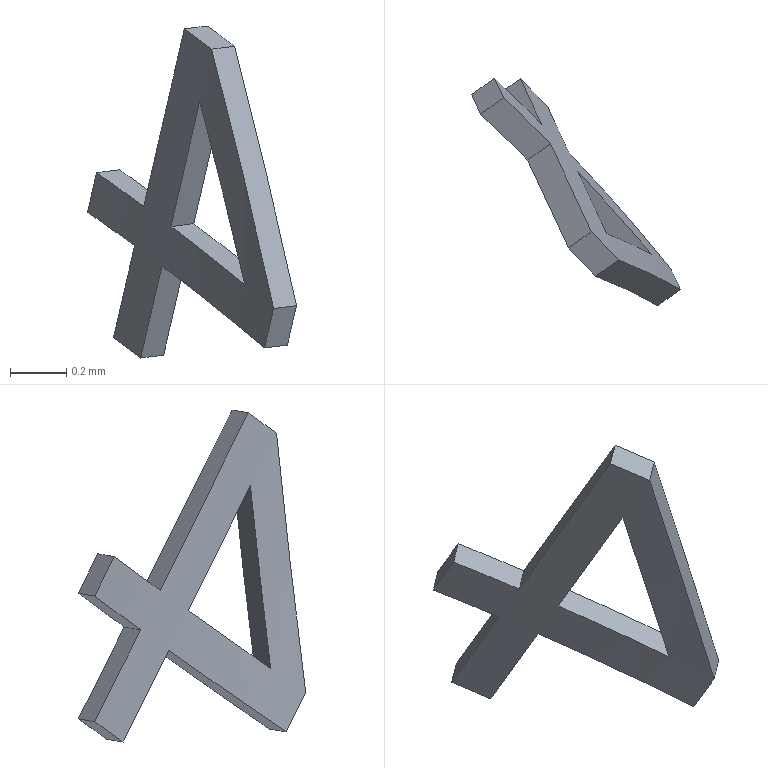Part | SolidWorks | features BaseBody 1 | 1 solid | 16 faces | box 0.7417 x 0.8074 x 1.179 mm | volume 0.04503 mm3 | plane 14 | cylinder 2 | commonest cylinder face diameters 16.8 x1 17 x1
STEP:
#1=CARTESIAN_POINT('',(1972.672,-237.776,993.123));
#2=VERTEX_POINT('',#1);
#3=CARTESIAN_POINT('',(1972.747,-237.939,993.449));
#4=VERTEX_POINT('',#3);
#5=CARTESIAN_POINT('',(1973.875,-240.379,998.359));
#6=DIRECTION('',(0.2015,-0.436,0.8771));
#7=VECTOR('',#6,1000.);
#8=LINE('',#5,#7);
#9=EDGE_CURVE('',#2,#4,#8,.T.);
#10=ORIENTED_EDGE('',*,*,#9,.T.);
#11=CARTESIAN_POINT('',(1973.112,-238.355,993.158));
#12=VERTEX_POINT('',#11);
#13=CARTESIAN_POINT('',(1966.322,-243.225,992.297));
#14=DIRECTION('',(-0.2015,0.436,-0.8771));
#15=DIRECTION('',(-0.7309,-0.6631,-0.1618));
#16=AXIS2_PLACEMENT_3D('',#13,#14,#15);
#17=CIRCLE('',#16,8.4);
#18=EDGE_CURVE('',#4,#12,#17,.T.);
#19=ORIENTED_EDGE('',*,*,#18,.T.);
#20=CARTESIAN_POINT('',(1973.144,-238.425,993.298));
#21=VERTEX_POINT('',#20);
#22=CARTESIAN_POINT('',(1974.24,-240.796,998.068));
#23=DIRECTION('',(0.2015,-0.436,0.8771));
#24=VECTOR('',#23,1000.);
#25=LINE('',#22,#24);
#26=EDGE_CURVE('',#12,#21,#25,.T.);
#27=ORIENTED_EDGE('',*,*,#26,.T.);
#28=CARTESIAN_POINT('',(1972.924,-238.321,994.219));
#29=VERTEX_POINT('',#28);
#30=CARTESIAN_POINT('',(1972.924,-238.321,994.219));
#31=CARTESIAN_POINT('',(1973.004,-238.351,993.913));
#32=CARTESIAN_POINT('',(1973.077,-238.386,993.606));
#33=CARTESIAN_POINT('',(1973.144,-238.425,993.298));
#34=B_SPLINE_CURVE_WITH_KNOTS('',3,(#30,#31,#32,#33),.UNSPECIFIED.,.F.,.F.,(4,4),(0.,1.),.UNSPECIFIED.);
#35=EDGE_CURVE('',#29,#21,#34,.T.);
#36=ORIENTED_EDGE('',*,*,#35,.F.);
#37=CARTESIAN_POINT('',(1972.827,-238.221,994.291));
#38=VERTEX_POINT('',#37);
#39=CARTESIAN_POINT('',(1966.499,-243.608,993.067));
#40=DIRECTION('',(0.2015,-0.436,0.8771));
#41=DIRECTION('',(-0.7309,-0.6631,-0.1618));
#42=AXIS2_PLACEMENT_3D('',#39,#40,#41);
#43=CIRCLE('',#42,8.4);
#44=EDGE_CURVE('',#29,#38,#43,.T.);
#45=ORIENTED_EDGE('',*,*,#44,.T.);
#46=CARTESIAN_POINT('',(1972.683,-237.908,993.661));
#47=VERTEX_POINT('',#46);
#48=CARTESIAN_POINT('',(1973.778,-240.28,998.431));
#49=DIRECTION('',(-0.2015,0.436,-0.8771));
#50=VECTOR('',#49,1000.);
#51=LINE('',#48,#50);
#52=EDGE_CURVE('',#38,#47,#51,.T.);
#53=ORIENTED_EDGE('',*,*,#52,.T.);
#54=CARTESIAN_POINT('',(1972.515,-237.746,993.781));
#55=VERTEX_POINT('',#54);
#56=CARTESIAN_POINT('',(1966.354,-243.295,992.437));
#57=DIRECTION('',(0.2015,-0.436,0.8771));
#58=DIRECTION('',(-0.7309,-0.6631,-0.1618));
#59=AXIS2_PLACEMENT_3D('',#56,#57,#58);
#60=CIRCLE('',#59,8.4);
#61=EDGE_CURVE('',#47,#55,#60,.T.);
#62=ORIENTED_EDGE('',*,*,#61,.T.);
#63=CARTESIAN_POINT('',(1972.483,-237.676,993.641));
#64=VERTEX_POINT('',#63);
#65=CARTESIAN_POINT('',(1973.611,-240.117,998.55));
#66=DIRECTION('',(-0.2015,0.436,-0.8771));
#67=VECTOR('',#66,1000.);
#68=LINE('',#65,#67);
#69=EDGE_CURVE('',#55,#64,#68,.T.);
#70=ORIENTED_EDGE('',*,*,#69,.T.);
#71=CARTESIAN_POINT('',(1972.65,-237.839,993.521));
#72=VERTEX_POINT('',#71);
#73=CARTESIAN_POINT('',(1966.322,-243.225,992.297));
#74=DIRECTION('',(-0.2015,0.436,-0.8771));
#75=DIRECTION('',(-0.7309,-0.6631,-0.1618));
#76=AXIS2_PLACEMENT_3D('',#73,#74,#75);
#77=CIRCLE('',#76,8.4);
#78=EDGE_CURVE('',#64,#72,#77,.T.);
#79=ORIENTED_EDGE('',*,*,#78,.T.);
#80=CARTESIAN_POINT('',(1972.575,-237.676,993.195));
#81=VERTEX_POINT('',#80);
#82=CARTESIAN_POINT('',(1973.778,-240.28,998.431));
#83=DIRECTION('',(-0.2015,0.436,-0.8771));
#84=VECTOR('',#83,1000.);
#85=LINE('',#82,#84);
#86=EDGE_CURVE('',#72,#81,#85,.T.);
#87=ORIENTED_EDGE('',*,*,#86,.T.);
#88=CARTESIAN_POINT('',(1966.247,-243.063,991.97));
#89=DIRECTION('',(-0.2015,0.436,-0.8771));
#90=DIRECTION('',(-0.7309,-0.6631,-0.1618));
#91=AXIS2_PLACEMENT_3D('',#88,#89,#90);
#92=CIRCLE('',#91,8.4);
#93=EDGE_CURVE('',#81,#2,#92,.T.);
#94=ORIENTED_EDGE('',*,*,#93,.T.);
#95=EDGE_LOOP('',(#10,#19,#27,#36,#45,#53,#62,#70,#79,#87,#94));
#96=FACE_OUTER_BOUND('',#95,.T.);
#97=CARTESIAN_POINT('',(1972.881,-238.229,994.032));
#98=VERTEX_POINT('',#97);
#99=CARTESIAN_POINT('',(1973.042,-238.301,993.384));
#100=VERTEX_POINT('',#99);
#101=CARTESIAN_POINT('',(1972.881,-238.229,994.032));
#102=CARTESIAN_POINT('',(1972.938,-238.25,993.817));
#103=CARTESIAN_POINT('',(1972.991,-238.274,993.6));
#104=CARTESIAN_POINT('',(1973.042,-238.301,993.384));
#105=B_SPLINE_CURVE_WITH_KNOTS('',3,(#101,#102,#103,#104),.UNSPECIFIED.,.F.,.F.,(4,4),(0.,1.),.UNSPECIFIED.);
#106=EDGE_CURVE('',#98,#100,#105,.T.);
#107=ORIENTED_EDGE('',*,*,#106,.T.);
#108=CARTESIAN_POINT('',(1972.78,-238.008,993.589));
#109=VERTEX_POINT('',#108);
#110=CARTESIAN_POINT('',(1966.354,-243.295,992.437));
#111=DIRECTION('',(0.2015,-0.436,0.8771));
#112=DIRECTION('',(-0.7309,-0.6631,-0.1618));
#113=AXIS2_PLACEMENT_3D('',#110,#111,#112);
#114=CIRCLE('',#113,8.4);
#115=EDGE_CURVE('',#100,#109,#114,.T.);
#116=ORIENTED_EDGE('',*,*,#115,.T.);
#117=CARTESIAN_POINT('',(1973.875,-240.379,998.359));
#118=DIRECTION('',(0.2015,-0.436,0.8771));
#119=VECTOR('',#118,1000.);
#120=LINE('',#117,#119);
#121=EDGE_CURVE('',#109,#98,#120,.T.);
#122=ORIENTED_EDGE('',*,*,#121,.T.);
#123=EDGE_LOOP('',(#107,#116,#122));
#124=FACE_BOUND('',#123,.T.);
#125=CARTESIAN_POINT('',(1967.45,-245.666,997.207));
#126=DIRECTION('',(0.2015,-0.436,0.8771));
#127=DIRECTION('',(-0.7309,-0.6631,-0.1618));
#128=AXIS2_PLACEMENT_3D('',#125,#126,#127);
#129=CYLINDRICAL_SURFACE('',#128,8.4);
#130=ADVANCED_FACE('',(#96,#124),#129,.F.);
#131=CARTESIAN_POINT('',(1972.754,-237.718,993.133));
#132=VERTEX_POINT('',#131);
#133=CARTESIAN_POINT('',(1972.713,-237.747,993.128));
#134=DIRECTION('',(-0.8088,-0.5792,-0.1022));
#135=VECTOR('',#134,1000.);
#136=LINE('',#133,#135);
#137=EDGE_CURVE('',#132,#2,#136,.T.);
#138=ORIENTED_EDGE('',*,*,#137,.T.);
#139=ORIENTED_EDGE('',*,*,#93,.F.);
#140=CARTESIAN_POINT('',(1972.657,-237.618,993.205));
#141=VERTEX_POINT('',#140);
#142=CARTESIAN_POINT('',(1972.616,-237.647,993.2));
#143=DIRECTION('',(-0.8088,-0.5792,-0.1022));
#144=VECTOR('',#143,1000.);
#145=LINE('',#142,#144);
#146=EDGE_CURVE('',#141,#81,#145,.T.);
#147=ORIENTED_EDGE('',*,*,#146,.F.);
#148=CARTESIAN_POINT('',(1966.247,-243.063,991.97));
#149=DIRECTION('',(-0.2015,0.436,-0.8771));
#150=DIRECTION('',(-0.7309,-0.6631,-0.1618));
#151=AXIS2_PLACEMENT_3D('',#148,#149,#150);
#152=CIRCLE('',#151,8.5);
#153=EDGE_CURVE('',#141,#132,#152,.T.);
#154=ORIENTED_EDGE('',*,*,#153,.T.);
#155=EDGE_LOOP('',(#138,#139,#147,#154));
#156=FACE_OUTER_BOUND('',#155,.T.);
#157=CARTESIAN_POINT('',(1981.656,-238.46,990.719));
#158=DIRECTION('',(-0.2015,0.436,-0.8771));
#159=DIRECTION('',(-0.5526,0.6888,0.4693));
#160=AXIS2_PLACEMENT_3D('',#157,#158,#159);
#161=PLANE('',#160);
#162=ADVANCED_FACE('',(#156),#161,.T.);
#163=ORIENTED_EDGE('',*,*,#146,.T.);
#164=ORIENTED_EDGE('',*,*,#86,.F.);
#165=CARTESIAN_POINT('',(1972.732,-237.781,993.532));
#166=VERTEX_POINT('',#165);
#167=CARTESIAN_POINT('',(1972.691,-237.81,993.526));
#168=DIRECTION('',(-0.8088,-0.5792,-0.1022));
#169=VECTOR('',#168,1000.);
#170=LINE('',#167,#169);
#171=EDGE_CURVE('',#166,#72,#170,.T.);
#172=ORIENTED_EDGE('',*,*,#171,.F.);
#173=CARTESIAN_POINT('',(1972.694,-237.699,993.368));
#174=DIRECTION('',(-0.2015,0.436,-0.8771));
#175=VECTOR('',#174,1000.);
#176=LINE('',#173,#175);
#177=EDGE_CURVE('',#166,#141,#176,.T.);
#178=ORIENTED_EDGE('',*,*,#177,.T.);
#179=EDGE_LOOP('',(#163,#164,#172,#178));
#180=FACE_OUTER_BOUND('',#179,.T.);
#181=CARTESIAN_POINT('',(1978.018,-233.995,994.199));
#182=DIRECTION('',(-0.5526,0.6888,0.4693));
#183=DIRECTION('',(0.2015,-0.436,0.8771));
#184=AXIS2_PLACEMENT_3D('',#181,#182,#183);
#185=PLANE('',#184);
#186=ADVANCED_FACE('',(#180),#185,.T.);
#187=ORIENTED_EDGE('',*,*,#171,.T.);
#188=ORIENTED_EDGE('',*,*,#78,.F.);
#189=CARTESIAN_POINT('',(1972.565,-237.618,993.651));
#190=VERTEX_POINT('',#189);
#191=CARTESIAN_POINT('',(1972.524,-237.647,993.646));
#192=DIRECTION('',(-0.8088,-0.5792,-0.1022));
#193=VECTOR('',#192,1000.);
#194=LINE('',#191,#193);
#195=EDGE_CURVE('',#190,#64,#194,.T.);
#196=ORIENTED_EDGE('',*,*,#195,.F.);
#197=CARTESIAN_POINT('',(1966.322,-243.225,992.297));
#198=DIRECTION('',(-0.2015,0.436,-0.8771));
#199=DIRECTION('',(-0.7309,-0.6631,-0.1618));
#200=AXIS2_PLACEMENT_3D('',#197,#198,#199);
#201=CIRCLE('',#200,8.5);
#202=EDGE_CURVE('',#190,#166,#201,.T.);
#203=ORIENTED_EDGE('',*,*,#202,.T.);
#204=EDGE_LOOP('',(#187,#188,#196,#203));
#205=FACE_OUTER_BOUND('',#204,.T.);
#206=CARTESIAN_POINT('',(1977.874,-233.815,994.322));
#207=DIRECTION('',(-0.2015,0.436,-0.8771));
#208=DIRECTION('',(-0.5526,0.6888,0.4693));
#209=AXIS2_PLACEMENT_3D('',#206,#207,#208);
#210=PLANE('',#209);
#211=ADVANCED_FACE('',(#205),#210,.T.);
#212=ORIENTED_EDGE('',*,*,#195,.T.);
#213=ORIENTED_EDGE('',*,*,#69,.F.);
#214=CARTESIAN_POINT('',(1972.597,-237.687,993.791));
#215=VERTEX_POINT('',#214);
#216=CARTESIAN_POINT('',(1972.556,-237.716,993.786));
#217=DIRECTION('',(-0.8088,-0.5792,-0.1022));
#218=VECTOR('',#217,1000.);
#219=LINE('',#216,#218);
#220=EDGE_CURVE('',#215,#55,#219,.T.);
#221=ORIENTED_EDGE('',*,*,#220,.F.);
#222=CARTESIAN_POINT('',(1972.581,-237.652,993.721));
#223=DIRECTION('',(-0.2015,0.436,-0.8771));
#224=VECTOR('',#223,1000.);
#225=LINE('',#222,#224);
#226=EDGE_CURVE('',#215,#190,#225,.T.);
#227=ORIENTED_EDGE('',*,*,#226,.T.);
#228=EDGE_LOOP('',(#212,#213,#221,#227));
#229=FACE_OUTER_BOUND('',#228,.T.);
#230=CARTESIAN_POINT('',(1977.906,-233.885,994.462));
#231=DIRECTION('',(-0.5526,0.6888,0.4693));
#232=DIRECTION('',(0.2015,-0.436,0.8771));
#233=AXIS2_PLACEMENT_3D('',#230,#231,#232);
#234=PLANE('',#233);
#235=ADVANCED_FACE('',(#229),#234,.T.);
#236=ORIENTED_EDGE('',*,*,#220,.T.);
#237=ORIENTED_EDGE('',*,*,#61,.F.);
#238=CARTESIAN_POINT('',(1972.764,-237.85,993.671));
#239=VERTEX_POINT('',#238);
#240=CARTESIAN_POINT('',(1972.723,-237.879,993.666));
#241=DIRECTION('',(-0.8088,-0.5792,-0.1022));
#242=VECTOR('',#241,1000.);
#243=LINE('',#240,#242);
#244=EDGE_CURVE('',#239,#47,#243,.T.);
#245=ORIENTED_EDGE('',*,*,#244,.F.);
#246=CARTESIAN_POINT('',(1966.354,-243.295,992.437));
#247=DIRECTION('',(0.2015,-0.436,0.8771));
#248=DIRECTION('',(-0.7309,-0.6631,-0.1618));
#249=AXIS2_PLACEMENT_3D('',#246,#247,#248);
#250=CIRCLE('',#249,8.5);
#251=EDGE_CURVE('',#239,#215,#250,.T.);
#252=ORIENTED_EDGE('',*,*,#251,.T.);
#253=EDGE_LOOP('',(#236,#237,#245,#252));
#254=FACE_OUTER_BOUND('',#253,.T.);
#255=CARTESIAN_POINT('',(1978.05,-234.064,994.339));
#256=DIRECTION('',(0.2015,-0.436,0.8771));
#257=DIRECTION('',(0.5526,-0.6888,-0.4693));
#258=AXIS2_PLACEMENT_3D('',#255,#256,#257);
#259=PLANE('',#258);
#260=ADVANCED_FACE('',(#254),#259,.T.);
#261=ORIENTED_EDGE('',*,*,#244,.T.);
#262=ORIENTED_EDGE('',*,*,#52,.F.);
#263=CARTESIAN_POINT('',(1972.908,-238.163,994.301));
#264=VERTEX_POINT('',#263);
#265=CARTESIAN_POINT('',(1972.868,-238.192,994.296));
#266=DIRECTION('',(-0.8088,-0.5792,-0.1022));
#267=VECTOR('',#266,1000.);
#268=LINE('',#265,#267);
#269=EDGE_CURVE('',#264,#38,#268,.T.);
#270=ORIENTED_EDGE('',*,*,#269,.F.);
#271=CARTESIAN_POINT('',(1972.836,-238.007,993.986));
#272=DIRECTION('',(-0.2015,0.436,-0.8771));
#273=VECTOR('',#272,1000.);
#274=LINE('',#271,#273);
#275=EDGE_CURVE('',#264,#239,#274,.T.);
#276=ORIENTED_EDGE('',*,*,#275,.T.);
#277=EDGE_LOOP('',(#261,#262,#270,#276));
#278=FACE_OUTER_BOUND('',#277,.T.);
#279=CARTESIAN_POINT('',(1978.018,-233.995,994.199));
#280=DIRECTION('',(-0.5526,0.6888,0.4693));
#281=DIRECTION('',(0.2015,-0.436,0.8771));
#282=AXIS2_PLACEMENT_3D('',#279,#280,#281);
#283=PLANE('',#282);
#284=ADVANCED_FACE('',(#278),#283,.T.);
#285=ORIENTED_EDGE('',*,*,#269,.T.);
#286=ORIENTED_EDGE('',*,*,#44,.F.);
#287=CARTESIAN_POINT('',(1973.005,-238.263,994.229));
#288=VERTEX_POINT('',#287);
#289=CARTESIAN_POINT('',(1972.965,-238.292,994.224));
#290=DIRECTION('',(-0.8088,-0.5792,-0.1022));
#291=VECTOR('',#290,1000.);
#292=LINE('',#289,#291);
#293=EDGE_CURVE('',#288,#29,#292,.T.);
#294=ORIENTED_EDGE('',*,*,#293,.F.);
#295=CARTESIAN_POINT('',(1966.499,-243.608,993.067));
#296=DIRECTION('',(0.2015,-0.436,0.8771));
#297=DIRECTION('',(-0.7309,-0.6631,-0.1618));
#298=AXIS2_PLACEMENT_3D('',#295,#296,#297);
#299=CIRCLE('',#298,8.5);
#300=EDGE_CURVE('',#288,#264,#299,.T.);
#301=ORIENTED_EDGE('',*,*,#300,.T.);
#302=EDGE_LOOP('',(#285,#286,#294,#301));
#303=FACE_OUTER_BOUND('',#302,.T.);
#304=CARTESIAN_POINT('',(1982.253,-239.435,991.522));
#305=DIRECTION('',(0.2015,-0.436,0.8771));
#306=DIRECTION('',(0.5526,-0.6888,-0.4693));
#307=AXIS2_PLACEMENT_3D('',#304,#305,#306);
#308=PLANE('',#307);
#309=ADVANCED_FACE('',(#303),#308,.T.);
#310=ORIENTED_EDGE('',*,*,#293,.T.);
#311=ORIENTED_EDGE('',*,*,#35,.T.);
#312=CARTESIAN_POINT('',(1973.225,-238.367,993.309));
#313=VERTEX_POINT('',#312);
#314=CARTESIAN_POINT('',(1973.185,-238.396,993.303));
#315=DIRECTION('',(-0.8088,-0.5792,-0.1022));
#316=VECTOR('',#315,1000.);
#317=LINE('',#314,#316);
#318=EDGE_CURVE('',#313,#21,#317,.T.);
#319=ORIENTED_EDGE('',*,*,#318,.F.);
#320=CARTESIAN_POINT('',(1973.005,-238.263,994.229));
#321=CARTESIAN_POINT('',(1973.053,-238.281,994.046));
#322=CARTESIAN_POINT('',(1973.099,-238.301,993.862));
#323=CARTESIAN_POINT('',(1973.143,-238.322,993.678));
#324=CARTESIAN_POINT('',(1973.185,-238.344,993.493));
#325=CARTESIAN_POINT('',(1973.225,-238.367,993.309));
#326=B_SPLINE_CURVE_WITH_KNOTS('',5,(#320,#321,#322,#323,#324,#325),.UNSPECIFIED.,.F.,.F.,(6,6),(0.,1.),.UNSPECIFIED.);
#327=EDGE_CURVE('',#288,#313,#326,.T.);
#328=ORIENTED_EDGE('',*,*,#327,.F.);
#329=EDGE_LOOP('',(#310,#311,#319,#328));
#330=FACE_OUTER_BOUND('',#329,.T.);
#331=CARTESIAN_POINT('',(1978.482,-234.602,993.973));
#332=DIRECTION('',(0.5491,-0.8058,0.2218));
#333=DIRECTION('',(0.2108,-0.1233,-0.9697));
#334=AXIS2_PLACEMENT_3D('',#331,#332,#333);
#335=PLANE('',#334);
#336=ADVANCED_FACE('',(#330),#335,.T.);
#337=ORIENTED_EDGE('',*,*,#318,.T.);
#338=ORIENTED_EDGE('',*,*,#26,.F.);
#339=CARTESIAN_POINT('',(1973.193,-238.297,993.169));
#340=VERTEX_POINT('',#339);
#341=CARTESIAN_POINT('',(1973.152,-238.326,993.163));
#342=DIRECTION('',(-0.8088,-0.5792,-0.1022));
#343=VECTOR('',#342,1000.);
#344=LINE('',#341,#343);
#345=EDGE_CURVE('',#340,#12,#344,.T.);
#346=ORIENTED_EDGE('',*,*,#345,.F.);
#347=CARTESIAN_POINT('',(1973.209,-238.332,993.239));
#348=DIRECTION('',(0.2015,-0.436,0.8771));
#349=VECTOR('',#348,1000.);
#350=LINE('',#347,#349);
#351=EDGE_CURVE('',#340,#313,#350,.T.);
#352=ORIENTED_EDGE('',*,*,#351,.T.);
#353=EDGE_LOOP('',(#337,#338,#346,#352));
#354=FACE_OUTER_BOUND('',#353,.T.);
#355=CARTESIAN_POINT('',(1978.45,-234.533,993.833));
#356=DIRECTION('',(0.5526,-0.6888,-0.4693));
#357=DIRECTION('',(-0.2015,0.436,-0.8771));
#358=AXIS2_PLACEMENT_3D('',#355,#356,#357);
#359=PLANE('',#358);
#360=ADVANCED_FACE('',(#354),#359,.T.);
#361=ORIENTED_EDGE('',*,*,#345,.T.);
#362=ORIENTED_EDGE('',*,*,#18,.F.);
#363=CARTESIAN_POINT('',(1972.829,-237.881,993.46));
#364=VERTEX_POINT('',#363);
#365=CARTESIAN_POINT('',(1972.788,-237.91,993.454));
#366=DIRECTION('',(-0.8088,-0.5792,-0.1022));
#367=VECTOR('',#366,1000.);
#368=LINE('',#365,#367);
#369=EDGE_CURVE('',#364,#4,#368,.T.);
#370=ORIENTED_EDGE('',*,*,#369,.F.);
#371=CARTESIAN_POINT('',(1966.322,-243.225,992.297));
#372=DIRECTION('',(-0.2015,0.436,-0.8771));
#373=DIRECTION('',(-0.7309,-0.6631,-0.1618));
#374=AXIS2_PLACEMENT_3D('',#371,#372,#373);
#375=CIRCLE('',#374,8.5);
#376=EDGE_CURVE('',#364,#340,#375,.T.);
#377=ORIENTED_EDGE('',*,*,#376,.T.);
#378=EDGE_LOOP('',(#361,#362,#370,#377));
#379=FACE_OUTER_BOUND('',#378,.T.);
#380=CARTESIAN_POINT('',(1977.874,-233.815,994.322));
#381=DIRECTION('',(-0.2015,0.436,-0.8771));
#382=DIRECTION('',(-0.5526,0.6888,0.4693));
#383=AXIS2_PLACEMENT_3D('',#380,#381,#382);
#384=PLANE('',#383);
#385=ADVANCED_FACE('',(#379),#384,.T.);
#386=ORIENTED_EDGE('',*,*,#369,.T.);
#387=ORIENTED_EDGE('',*,*,#9,.F.);
#388=ORIENTED_EDGE('',*,*,#137,.F.);
#389=CARTESIAN_POINT('',(1972.791,-237.799,993.296));
#390=DIRECTION('',(0.2015,-0.436,0.8771));
#391=VECTOR('',#390,1000.);
#392=LINE('',#389,#391);
#393=EDGE_CURVE('',#132,#364,#392,.T.);
#394=ORIENTED_EDGE('',*,*,#393,.T.);
#395=EDGE_LOOP('',(#386,#387,#388,#394));
#396=FACE_OUTER_BOUND('',#395,.T.);
#397=CARTESIAN_POINT('',(1978.029,-233.94,993.8));
#398=DIRECTION('',(0.5526,-0.6888,-0.4693));
#399=DIRECTION('',(-0.2015,0.436,-0.8771));
#400=AXIS2_PLACEMENT_3D('',#397,#398,#399);
#401=PLANE('',#400);
#402=ADVANCED_FACE('',(#396),#401,.T.);
#403=CARTESIAN_POINT('',(1972.962,-238.171,994.043));
#404=VERTEX_POINT('',#403);
#405=CARTESIAN_POINT('',(1972.922,-238.2,994.038));
#406=DIRECTION('',(-0.8088,-0.5792,-0.1022));
#407=VECTOR('',#406,1000.);
#408=LINE('',#405,#407);
#409=EDGE_CURVE('',#404,#98,#408,.T.);
#410=ORIENTED_EDGE('',*,*,#409,.T.);
#411=ORIENTED_EDGE('',*,*,#121,.F.);
#412=CARTESIAN_POINT('',(1972.861,-237.95,993.599));
#413=VERTEX_POINT('',#412);
#414=CARTESIAN_POINT('',(1972.82,-237.979,993.594));
#415=DIRECTION('',(-0.8088,-0.5792,-0.1022));
#416=VECTOR('',#415,1000.);
#417=LINE('',#414,#416);
#418=EDGE_CURVE('',#413,#109,#417,.T.);
#419=ORIENTED_EDGE('',*,*,#418,.F.);
#420=CARTESIAN_POINT('',(1972.912,-238.06,993.821));
#421=DIRECTION('',(0.2015,-0.436,0.8771));
#422=VECTOR('',#421,1000.);
#423=LINE('',#420,#422);
#424=EDGE_CURVE('',#413,#404,#423,.T.);
#425=ORIENTED_EDGE('',*,*,#424,.T.);
#426=EDGE_LOOP('',(#410,#411,#419,#425));
#427=FACE_OUTER_BOUND('',#426,.T.);
#428=CARTESIAN_POINT('',(1978.029,-233.94,993.8));
#429=DIRECTION('',(0.5526,-0.6888,-0.4693));
#430=DIRECTION('',(-0.2015,0.436,-0.8771));
#431=AXIS2_PLACEMENT_3D('',#428,#429,#430);
#432=PLANE('',#431);
#433=ADVANCED_FACE('',(#427),#432,.T.);
#434=ORIENTED_EDGE('',*,*,#418,.T.);
#435=ORIENTED_EDGE('',*,*,#115,.F.);
#436=CARTESIAN_POINT('',(1973.123,-238.243,993.394));
#437=VERTEX_POINT('',#436);
#438=CARTESIAN_POINT('',(1973.082,-238.272,993.389));
#439=DIRECTION('',(-0.8088,-0.5792,-0.1022));
#440=VECTOR('',#439,1000.);
#441=LINE('',#438,#440);
#442=EDGE_CURVE('',#437,#100,#441,.T.);
#443=ORIENTED_EDGE('',*,*,#442,.F.);
#444=CARTESIAN_POINT('',(1966.354,-243.295,992.437));
#445=DIRECTION('',(0.2015,-0.436,0.8771));
#446=DIRECTION('',(-0.7309,-0.6631,-0.1618));
#447=AXIS2_PLACEMENT_3D('',#444,#445,#446);
#448=CIRCLE('',#447,8.5);
#449=EDGE_CURVE('',#437,#413,#448,.T.);
#450=ORIENTED_EDGE('',*,*,#449,.T.);
#451=EDGE_LOOP('',(#434,#435,#443,#450));
#452=FACE_OUTER_BOUND('',#451,.T.);
#453=CARTESIAN_POINT('',(1978.05,-234.064,994.339));
#454=DIRECTION('',(0.2015,-0.436,0.8771));
#455=DIRECTION('',(0.5526,-0.6888,-0.4693));
#456=AXIS2_PLACEMENT_3D('',#453,#454,#455);
#457=PLANE('',#456);
#458=ADVANCED_FACE('',(#452),#457,.T.);
#459=CARTESIAN_POINT('',(1972.962,-238.171,994.043));
#460=CARTESIAN_POINT('',(1972.996,-238.184,993.913));
#461=CARTESIAN_POINT('',(1973.029,-238.197,993.784));
#462=CARTESIAN_POINT('',(1973.061,-238.212,993.654));
#463=CARTESIAN_POINT('',(1973.092,-238.227,993.524));
#464=CARTESIAN_POINT('',(1973.123,-238.243,993.394));
#465=B_SPLINE_CURVE_WITH_KNOTS('',5,(#459,#460,#461,#462,#463,#464),.UNSPECIFIED.,.F.,.F.,(6,6),(0.,1.),.UNSPECIFIED.);
#466=EDGE_CURVE('',#404,#437,#465,.T.);
#467=ORIENTED_EDGE('',*,*,#466,.T.);
#468=ORIENTED_EDGE('',*,*,#442,.T.);
#469=ORIENTED_EDGE('',*,*,#106,.F.);
#470=ORIENTED_EDGE('',*,*,#409,.F.);
#471=EDGE_LOOP('',(#467,#468,#469,#470));
#472=FACE_OUTER_BOUND('',#471,.T.);
#473=CARTESIAN_POINT('',(1978.381,-234.477,994.058));
#474=DIRECTION('',(0.5484,-0.8054,0.225));
#475=DIRECTION('',(0.2126,-0.1259,-0.969));
#476=AXIS2_PLACEMENT_3D('',#473,#474,#475);
#477=PLANE('',#476);
#478=ADVANCED_FACE('',(#472),#477,.F.);
#479=ORIENTED_EDGE('',*,*,#153,.F.);
#480=ORIENTED_EDGE('',*,*,#177,.F.);
#481=ORIENTED_EDGE('',*,*,#202,.F.);
#482=ORIENTED_EDGE('',*,*,#226,.F.);
#483=ORIENTED_EDGE('',*,*,#251,.F.);
#484=ORIENTED_EDGE('',*,*,#275,.F.);
#485=ORIENTED_EDGE('',*,*,#300,.F.);
#486=ORIENTED_EDGE('',*,*,#327,.T.);
#487=ORIENTED_EDGE('',*,*,#351,.F.);
#488=ORIENTED_EDGE('',*,*,#376,.F.);
#489=ORIENTED_EDGE('',*,*,#393,.F.);
#490=EDGE_LOOP('',(#479,#480,#481,#482,#483,#484,#485,#486,#487,#488,#489));
#491=FACE_OUTER_BOUND('',#490,.T.);
#492=ORIENTED_EDGE('',*,*,#466,.F.);
#493=ORIENTED_EDGE('',*,*,#424,.F.);
#494=ORIENTED_EDGE('',*,*,#449,.F.);
#495=EDGE_LOOP('',(#492,#493,#494));
#496=FACE_BOUND('',#495,.T.);
#497=CARTESIAN_POINT('',(1967.45,-245.666,997.207));
#498=DIRECTION('',(0.2015,-0.436,0.8771));
#499=DIRECTION('',(-0.7309,-0.6631,-0.1618));
#500=AXIS2_PLACEMENT_3D('',#497,#498,#499);
#501=CYLINDRICAL_SURFACE('',#500,8.5);
#502=ADVANCED_FACE('',(#491,#496),#501,.T.);
#503=CLOSED_SHELL('',(#130,#162,#186,#211,#235,#260,#284,#309,#336,#360,#385,#402,#433,#458,#478,#502));
#504=MANIFOLD_SOLID_BREP('',#503);
#505=CARTESIAN_POINT('',(0.,0.,0.));
#506=DIRECTION('',(0.,0.,1.));
#507=DIRECTION('',(1.,0.,0.));
#508=AXIS2_PLACEMENT_3D('',#505,#506,#507);
#509=(LENGTH_UNIT()NAMED_UNIT(*)SI_UNIT(.MILLI.,.METRE.));
#510=UNCERTAINTY_MEASURE_WITH_UNIT(LENGTH_MEASURE(0.00001),#509,'','');
#511=(NAMED_UNIT(*)PLANE_ANGLE_UNIT()SI_UNIT($,.RADIAN.));
#512=(NAMED_UNIT(*)SI_UNIT($,.STERADIAN.)SOLID_ANGLE_UNIT());
#513=(GEOMETRIC_REPRESENTATION_CONTEXT(3)GLOBAL_UNCERTAINTY_ASSIGNED_CONTEXT((#510))GLOBAL_UNIT_ASSIGNED_CONTEXT((#509,#511,#512))REPRESENTATION_CONTEXT('',''));
#514=ADVANCED_BREP_SHAPE_REPRESENTATION('',(#504,#508),#513);